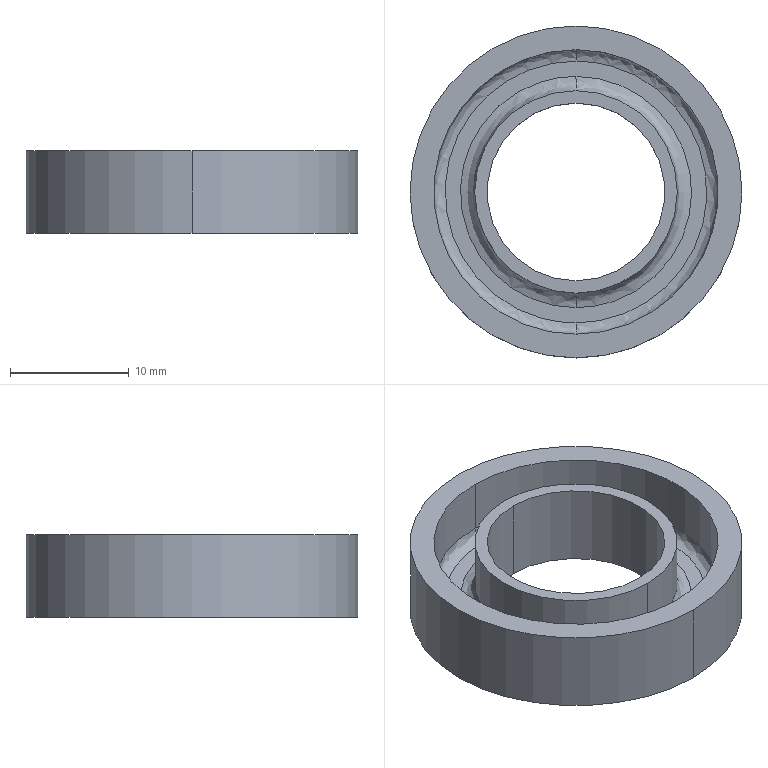Part | SolidWorks | features BaseBody 1 | 1 solid | 16 faces | box 28 x 28 x 7 mm | volume 1879 mm3 | cylinder 8 | spline 4 | plane 4 | commonest cylinder face diameters 15 x2 17.088 x2 24 x2 28 x2
STEP:
#1=CARTESIAN_POINT('',(0.,-11.038,1.5));
#2=VERTEX_POINT('',#1);
#3=CARTESIAN_POINT('',(0.,11.038,1.5));
#4=VERTEX_POINT('',#3);
#5=CARTESIAN_POINT('',(0.,-11.038,1.5));
#6=CARTESIAN_POINT('',(0.3374,-11.038,1.5));
#7=CARTESIAN_POINT('',(0.8415,-11.015,1.5));
#8=CARTESIAN_POINT('',(1.426,-10.948,1.5));
#9=CARTESIAN_POINT('',(1.718,-10.904,1.5));
#10=CARTESIAN_POINT('',(1.863,-10.879,1.5));
#11=CARTESIAN_POINT('',(1.925,-10.869,1.5));
#12=CARTESIAN_POINT('',(1.967,-10.861,1.5));
#13=CARTESIAN_POINT('',(1.986,-10.858,1.5));
#14=CARTESIAN_POINT('',(2.36,-10.788,1.5));
#15=CARTESIAN_POINT('',(2.881,-10.666,1.5));
#16=CARTESIAN_POINT('',(3.476,-10.479,1.5));
#17=CARTESIAN_POINT('',(3.771,-10.374,1.5));
#18=CARTESIAN_POINT('',(3.896,-10.327,1.5));
#19=CARTESIAN_POINT('',(3.98,-10.295,1.5));
#20=CARTESIAN_POINT('',(4.02,-10.28,1.5));
#21=CARTESIAN_POINT('',(4.41,-10.126,1.5));
#22=CARTESIAN_POINT('',(4.917,-9.895,1.5));
#23=CARTESIAN_POINT('',(5.486,-9.581,1.5));
#24=CARTESIAN_POINT('',(5.725,-9.437,1.5));
#25=CARTESIAN_POINT('',(5.883,-9.34,1.5));
#26=CARTESIAN_POINT('',(5.96,-9.291,1.5));
#27=CARTESIAN_POINT('',(6.677,-8.822,1.5));
#28=CARTESIAN_POINT('',(7.266,-8.343,1.5));
#29=CARTESIAN_POINT('',(8.074,-7.536,1.5));
#30=CARTESIAN_POINT('',(8.455,-7.113,1.5));
#31=CARTESIAN_POINT('',(8.86,-6.587,1.5));
#32=CARTESIAN_POINT('',(9.025,-6.355,1.5));
#33=CARTESIAN_POINT('',(9.133,-6.199,1.5));
#34=CARTESIAN_POINT('',(9.188,-6.118,1.5));
#35=CARTESIAN_POINT('',(9.443,-5.728,1.5));
#36=CARTESIAN_POINT('',(9.724,-5.247,1.5));
#37=CARTESIAN_POINT('',(10.008,-4.662,1.5));
#38=CARTESIAN_POINT('',(10.139,-4.365,1.5));
#39=CARTESIAN_POINT('',(10.193,-4.236,1.5));
#40=CARTESIAN_POINT('',(10.228,-4.15,1.5));
#41=CARTESIAN_POINT('',(10.246,-4.105,1.5));
#42=CARTESIAN_POINT('',(10.394,-3.73,1.5));
#43=CARTESIAN_POINT('',(10.567,-3.224,1.5));
#44=CARTESIAN_POINT('',(10.725,-2.62,1.5));
#45=CARTESIAN_POINT('',(10.793,-2.316,1.5));
#46=CARTESIAN_POINT('',(10.824,-2.162,1.5));
#47=CARTESIAN_POINT('',(10.837,-2.096,1.5));
#48=CARTESIAN_POINT('',(10.845,-2.052,1.5));
#49=CARTESIAN_POINT('',(10.85,-2.029,1.5));
#50=CARTESIAN_POINT('',(10.976,-1.345,1.5));
#51=CARTESIAN_POINT('',(11.038,-0.6753,1.5));
#52=CARTESIAN_POINT('',(11.038,0.3376,1.5));
#53=CARTESIAN_POINT('',(11.022,0.6736,1.5));
#54=CARTESIAN_POINT('',(10.976,1.176,1.5));
#55=CARTESIAN_POINT('',(10.947,1.426,1.5));
#56=CARTESIAN_POINT('',(10.904,1.718,1.5));
#57=CARTESIAN_POINT('',(10.879,1.863,1.5));
#58=CARTESIAN_POINT('',(10.868,1.925,1.5));
#59=CARTESIAN_POINT('',(10.861,1.967,1.5));
#60=CARTESIAN_POINT('',(10.858,1.986,1.5));
#61=CARTESIAN_POINT('',(10.788,2.36,1.5));
#62=CARTESIAN_POINT('',(10.666,2.881,1.5));
#63=CARTESIAN_POINT('',(10.479,3.476,1.5));
#64=CARTESIAN_POINT('',(10.374,3.771,1.5));
#65=CARTESIAN_POINT('',(10.327,3.896,1.5));
#66=CARTESIAN_POINT('',(10.295,3.98,1.5));
#67=CARTESIAN_POINT('',(10.28,4.02,1.5));
#68=CARTESIAN_POINT('',(10.126,4.41,1.5));
#69=CARTESIAN_POINT('',(9.895,4.917,1.5));
#70=CARTESIAN_POINT('',(9.581,5.486,1.5));
#71=CARTESIAN_POINT('',(9.437,5.725,1.5));
#72=CARTESIAN_POINT('',(9.34,5.883,1.5));
#73=CARTESIAN_POINT('',(9.291,5.96,1.5));
#74=CARTESIAN_POINT('',(8.822,6.677,1.5));
#75=CARTESIAN_POINT('',(8.343,7.266,1.5));
#76=CARTESIAN_POINT('',(7.536,8.074,1.5));
#77=CARTESIAN_POINT('',(7.113,8.455,1.5));
#78=CARTESIAN_POINT('',(6.587,8.86,1.5));
#79=CARTESIAN_POINT('',(6.355,9.025,1.5));
#80=CARTESIAN_POINT('',(6.199,9.133,1.5));
#81=CARTESIAN_POINT('',(6.118,9.188,1.5));
#82=CARTESIAN_POINT('',(5.728,9.443,1.5));
#83=CARTESIAN_POINT('',(5.247,9.724,1.5));
#84=CARTESIAN_POINT('',(4.662,10.008,1.5));
#85=CARTESIAN_POINT('',(4.365,10.139,1.5));
#86=CARTESIAN_POINT('',(4.236,10.193,1.5));
#87=CARTESIAN_POINT('',(4.15,10.228,1.5));
#88=CARTESIAN_POINT('',(4.105,10.246,1.5));
#89=CARTESIAN_POINT('',(3.73,10.394,1.5));
#90=CARTESIAN_POINT('',(3.224,10.567,1.5));
#91=CARTESIAN_POINT('',(2.62,10.725,1.5));
#92=CARTESIAN_POINT('',(2.316,10.793,1.5));
#93=CARTESIAN_POINT('',(2.162,10.824,1.5));
#94=CARTESIAN_POINT('',(2.096,10.837,1.5));
#95=CARTESIAN_POINT('',(2.052,10.845,1.5));
#96=CARTESIAN_POINT('',(2.029,10.85,1.5));
#97=CARTESIAN_POINT('',(1.345,10.976,1.5));
#98=CARTESIAN_POINT('',(0.6748,11.038,1.5));
#99=CARTESIAN_POINT('',(0.,11.038,1.5));
#100=B_SPLINE_CURVE_WITH_KNOTS('',3,(#5,#6,#7,#8,#9,#10,#11,#12,#13,#14,#15,#16,#17,#18,#19,#20,#21,#22,#23,#24,#25,#26,#27,#28,#29,#30,#31,#32,#33,#34,#35,#36,#37,#38,#39,#40,#41,#42,#43,#44,#45,#46,#47,#48,#49,#50,#51,#52,#53,#54,#55,#56,#57,#58,#59,#60,#61,#62,#63,#64,#65,#66,#67,#68,#69,#70,#71,#72,#73,#74,#75,#76,#77,#78,#79,#80,#81,#82,#83,#84,#85,#86,#87,#88,#89,#90,#91,#92,#93,#94,#95,#96,#97,#98,#99),.UNSPECIFIED.,.F.,.F.,(4,1,1,1,1,2,2,1,1,1,2,2,1,1,2,2,2,1,1,2,2,1,1,1,2,2,1,1,1,1,2,2,2,2,1,1,1,2,2,1,1,1,2,2,1,1,2,2,2,1,1,2,2,1,1,1,2,2,1,1,1,1,2,2,4),(0.75,0.7656,0.7734,0.7773,0.7793,0.7803,0.7812,0.7969,0.8047,0.8086,0.8105,0.8125,0.8281,0.8359,0.8398,0.8438,0.875,0.8906,0.8984,0.9023,0.9063,0.9219,0.9297,0.9336,0.9355,0.9375,0.9531,0.9609,0.9648,0.9668,0.9678,0.9688,1.,1.016,1.023,1.027,1.029,1.03,1.031,1.047,1.055,1.059,1.061,1.063,1.078,1.086,1.09,1.094,1.125,1.141,1.148,1.152,1.156,1.172,1.18,1.184,1.186,1.188,1.203,1.211,1.215,1.217,1.218,1.219,1.25),.UNSPECIFIED.);
#101=EDGE_CURVE('',#2,#4,#100,.T.);
#102=ORIENTED_EDGE('',*,*,#101,.F.);
#103=CARTESIAN_POINT('',(0.,-12.,2.462));
#104=VERTEX_POINT('',#103);
#105=CARTESIAN_POINT('',(0.,-11.038,2.462));
#106=DIRECTION('',(-1.,0.,0.));
#107=DIRECTION('',(0.,-1.,0.));
#108=AXIS2_PLACEMENT_3D('',#105,#106,#107);
#109=CIRCLE('',#108,0.9623);
#110=EDGE_CURVE('',#2,#104,#109,.T.);
#111=ORIENTED_EDGE('',*,*,#110,.T.);
#112=CARTESIAN_POINT('',(0.,12.,2.462));
#113=VERTEX_POINT('',#112);
#114=CARTESIAN_POINT('',(0.,0.,2.462));
#115=DIRECTION('',(0.,0.,1.));
#116=DIRECTION('',(0.,1.,0.));
#117=AXIS2_PLACEMENT_3D('',#114,#115,#116);
#118=CIRCLE('',#117,12.);
#119=EDGE_CURVE('',#104,#113,#118,.T.);
#120=ORIENTED_EDGE('',*,*,#119,.T.);
#121=CARTESIAN_POINT('',(0.,11.038,2.462));
#122=DIRECTION('',(1.,0.,0.));
#123=DIRECTION('',(0.,1.,0.));
#124=AXIS2_PLACEMENT_3D('',#121,#122,#123);
#125=CIRCLE('',#124,0.9623);
#126=EDGE_CURVE('',#4,#113,#125,.T.);
#127=ORIENTED_EDGE('',*,*,#126,.F.);
#128=EDGE_LOOP('',(#102,#111,#120,#127));
#129=FACE_OUTER_BOUND('',#128,.T.);
#130=CARTESIAN_POINT('',(0.,11.038,1.5));
#131=CARTESIAN_POINT('',(22.075,11.038,1.5));
#132=CARTESIAN_POINT('',(22.075,-11.038,1.5));
#133=CARTESIAN_POINT('',(0.,-11.038,1.5));
#134=CARTESIAN_POINT('',(0.,11.601,1.5));
#135=CARTESIAN_POINT('',(23.203,11.601,1.5));
#136=CARTESIAN_POINT('',(23.203,-11.601,1.5));
#137=CARTESIAN_POINT('',(0.,-11.601,1.5));
#138=CARTESIAN_POINT('',(0.,12.,1.899));
#139=CARTESIAN_POINT('',(24.,12.,1.899));
#140=CARTESIAN_POINT('',(24.,-12.,1.899));
#141=CARTESIAN_POINT('',(0.,-12.,1.899));
#142=CARTESIAN_POINT('',(0.,12.,2.462));
#143=CARTESIAN_POINT('',(24.,12.,2.462));
#144=CARTESIAN_POINT('',(24.,-12.,2.462));
#145=CARTESIAN_POINT('',(0.,-12.,2.462));
#146=(BOUNDED_SURFACE()B_SPLINE_SURFACE(3,3,((#130,#131,#132,#133),(#134,#135,#136,#137),(#138,#139,#140,#141),(#142,#143,#144,#145)),.UNSPECIFIED.,.F.,.F.,.T.)B_SPLINE_SURFACE_WITH_KNOTS((4,4),(4,4),(0.,1.),(0.,1.),.UNSPECIFIED.)GEOMETRIC_REPRESENTATION_ITEM()RATIONAL_B_SPLINE_SURFACE(((1.,0.3333,0.3333,1.),(0.8047,0.2682,0.2682,0.8047),(0.8047,0.2682,0.2682,0.8047),(1.,0.3333,0.3333,1.)))REPRESENTATION_ITEM('')SURFACE());
#147=ADVANCED_FACE('',(#129),#146,.F.);
#148=CARTESIAN_POINT('',(0.,-8.544,2.71));
#149=VERTEX_POINT('',#148);
#150=CARTESIAN_POINT('',(0.,8.544,2.71));
#151=VERTEX_POINT('',#150);
#152=CARTESIAN_POINT('',(0.,0.,2.71));
#153=DIRECTION('',(0.,0.,1.));
#154=DIRECTION('',(0.,1.,0.));
#155=AXIS2_PLACEMENT_3D('',#152,#153,#154);
#156=CIRCLE('',#155,8.544);
#157=EDGE_CURVE('',#149,#151,#156,.T.);
#158=ORIENTED_EDGE('',*,*,#157,.F.);
#159=CARTESIAN_POINT('',(0.,-9.755,1.5));
#160=VERTEX_POINT('',#159);
#161=CARTESIAN_POINT('',(0.,-9.755,2.71));
#162=DIRECTION('',(-1.,0.,0.));
#163=DIRECTION('',(0.,-1.,0.));
#164=AXIS2_PLACEMENT_3D('',#161,#162,#163);
#165=CIRCLE('',#164,1.21);
#166=EDGE_CURVE('',#149,#160,#165,.T.);
#167=ORIENTED_EDGE('',*,*,#166,.T.);
#168=CARTESIAN_POINT('',(0.,9.755,1.5));
#169=VERTEX_POINT('',#168);
#170=CARTESIAN_POINT('',(0.,9.755,1.5));
#171=CARTESIAN_POINT('',(0.2981,9.755,1.5));
#172=CARTESIAN_POINT('',(0.7436,9.734,1.5));
#173=CARTESIAN_POINT('',(1.26,9.675,1.5));
#174=CARTESIAN_POINT('',(1.518,9.636,1.5));
#175=CARTESIAN_POINT('',(1.628,9.618,1.5));
#176=CARTESIAN_POINT('',(1.702,9.605,1.5));
#177=CARTESIAN_POINT('',(1.736,9.599,1.5));
#178=CARTESIAN_POINT('',(2.086,9.534,1.5));
#179=CARTESIAN_POINT('',(2.546,9.426,1.5));
#180=CARTESIAN_POINT('',(3.072,9.261,1.5));
#181=CARTESIAN_POINT('',(3.332,9.168,1.5));
#182=CARTESIAN_POINT('',(3.443,9.127,1.5));
#183=CARTESIAN_POINT('',(3.517,9.099,1.5));
#184=CARTESIAN_POINT('',(3.552,9.085,1.5));
#185=CARTESIAN_POINT('',(3.897,8.948,1.5));
#186=CARTESIAN_POINT('',(4.345,8.744,1.5));
#187=CARTESIAN_POINT('',(4.848,8.467,1.5));
#188=CARTESIAN_POINT('',(5.059,8.34,1.5));
#189=CARTESIAN_POINT('',(5.199,8.254,1.5));
#190=CARTESIAN_POINT('',(5.267,8.211,1.5));
#191=CARTESIAN_POINT('',(5.901,7.796,1.5));
#192=CARTESIAN_POINT('',(6.422,7.373,1.5));
#193=CARTESIAN_POINT('',(7.135,6.66,1.5));
#194=CARTESIAN_POINT('',(7.472,6.286,1.5));
#195=CARTESIAN_POINT('',(7.83,5.822,1.5));
#196=CARTESIAN_POINT('',(7.976,5.616,1.5));
#197=CARTESIAN_POINT('',(8.071,5.478,1.5));
#198=CARTESIAN_POINT('',(8.119,5.407,1.5));
#199=CARTESIAN_POINT('',(8.345,5.062,1.5));
#200=CARTESIAN_POINT('',(8.593,4.637,1.5));
#201=CARTESIAN_POINT('',(8.844,4.12,1.5));
#202=CARTESIAN_POINT('',(8.96,3.857,1.5));
#203=CARTESIAN_POINT('',(9.008,3.743,1.5));
#204=CARTESIAN_POINT('',(9.039,3.667,1.5));
#205=CARTESIAN_POINT('',(9.055,3.627,1.5));
#206=CARTESIAN_POINT('',(9.186,3.297,1.5));
#207=CARTESIAN_POINT('',(9.339,2.849,1.5));
#208=CARTESIAN_POINT('',(9.478,2.316,1.5));
#209=CARTESIAN_POINT('',(9.538,2.046,1.5));
#210=CARTESIAN_POINT('',(9.566,1.911,1.5));
#211=CARTESIAN_POINT('',(9.577,1.853,1.5));
#212=CARTESIAN_POINT('',(9.584,1.814,1.5));
#213=CARTESIAN_POINT('',(9.588,1.793,1.5));
#214=CARTESIAN_POINT('',(9.7,1.188,1.5));
#215=CARTESIAN_POINT('',(9.755,0.5968,1.5));
#216=CARTESIAN_POINT('',(9.755,-0.2984,1.5));
#217=CARTESIAN_POINT('',(9.741,-0.5953,1.5));
#218=CARTESIAN_POINT('',(9.7,-1.039,1.5));
#219=CARTESIAN_POINT('',(9.675,-1.26,1.5));
#220=CARTESIAN_POINT('',(9.636,-1.518,1.5));
#221=CARTESIAN_POINT('',(9.618,-1.628,1.5));
#222=CARTESIAN_POINT('',(9.605,-1.702,1.5));
#223=CARTESIAN_POINT('',(9.599,-1.736,1.5));
#224=CARTESIAN_POINT('',(9.534,-2.086,1.5));
#225=CARTESIAN_POINT('',(9.426,-2.546,1.5));
#226=CARTESIAN_POINT('',(9.261,-3.072,1.5));
#227=CARTESIAN_POINT('',(9.168,-3.332,1.5));
#228=CARTESIAN_POINT('',(9.127,-3.443,1.5));
#229=CARTESIAN_POINT('',(9.099,-3.517,1.5));
#230=CARTESIAN_POINT('',(9.085,-3.552,1.5));
#231=CARTESIAN_POINT('',(8.948,-3.897,1.5));
#232=CARTESIAN_POINT('',(8.744,-4.345,1.5));
#233=CARTESIAN_POINT('',(8.467,-4.848,1.5));
#234=CARTESIAN_POINT('',(8.34,-5.059,1.5));
#235=CARTESIAN_POINT('',(8.254,-5.199,1.5));
#236=CARTESIAN_POINT('',(8.211,-5.267,1.5));
#237=CARTESIAN_POINT('',(7.796,-5.901,1.5));
#238=CARTESIAN_POINT('',(7.373,-6.422,1.5));
#239=CARTESIAN_POINT('',(6.66,-7.135,1.5));
#240=CARTESIAN_POINT('',(6.286,-7.472,1.5));
#241=CARTESIAN_POINT('',(5.822,-7.83,1.5));
#242=CARTESIAN_POINT('',(5.616,-7.976,1.5));
#243=CARTESIAN_POINT('',(5.478,-8.071,1.5));
#244=CARTESIAN_POINT('',(5.407,-8.119,1.5));
#245=CARTESIAN_POINT('',(5.062,-8.345,1.5));
#246=CARTESIAN_POINT('',(4.637,-8.593,1.5));
#247=CARTESIAN_POINT('',(4.12,-8.844,1.5));
#248=CARTESIAN_POINT('',(3.857,-8.96,1.5));
#249=CARTESIAN_POINT('',(3.743,-9.008,1.5));
#250=CARTESIAN_POINT('',(3.667,-9.039,1.5));
#251=CARTESIAN_POINT('',(3.627,-9.055,1.5));
#252=CARTESIAN_POINT('',(3.297,-9.186,1.5));
#253=CARTESIAN_POINT('',(2.849,-9.339,1.5));
#254=CARTESIAN_POINT('',(2.316,-9.478,1.5));
#255=CARTESIAN_POINT('',(2.046,-9.538,1.5));
#256=CARTESIAN_POINT('',(1.911,-9.566,1.5));
#257=CARTESIAN_POINT('',(1.853,-9.577,1.5));
#258=CARTESIAN_POINT('',(1.814,-9.584,1.5));
#259=CARTESIAN_POINT('',(1.793,-9.588,1.5));
#260=CARTESIAN_POINT('',(1.189,-9.7,1.5));
#261=CARTESIAN_POINT('',(0.5963,-9.754,1.5));
#262=CARTESIAN_POINT('',(0.,-9.755,1.5));
#263=B_SPLINE_CURVE_WITH_KNOTS('',3,(#170,#171,#172,#173,#174,#175,#176,#177,#178,#179,#180,#181,#182,#183,#184,#185,#186,#187,#188,#189,#190,#191,#192,#193,#194,#195,#196,#197,#198,#199,#200,#201,#202,#203,#204,#205,#206,#207,#208,#209,#210,#211,#212,#213,#214,#215,#216,#217,#218,#219,#220,#221,#222,#223,#224,#225,#226,#227,#228,#229,#230,#231,#232,#233,#234,#235,#236,#237,#238,#239,#240,#241,#242,#243,#244,#245,#246,#247,#248,#249,#250,#251,#252,#253,#254,#255,#256,#257,#258,#259,#260,#261,#262),.UNSPECIFIED.,.F.,.F.,(4,1,1,1,2,2,1,1,1,2,2,1,1,2,2,2,1,1,2,2,1,1,1,2,2,1,1,1,1,2,2,2,2,1,1,2,2,1,1,1,2,2,1,1,2,2,2,1,1,2,2,1,1,1,2,2,1,1,1,1,2,2,4),(0.75,0.7656,0.7734,0.7773,0.7793,0.7813,0.7969,0.8047,0.8086,0.8105,0.8125,0.8281,0.8359,0.8398,0.8438,0.875,0.8906,0.8984,0.9023,0.9063,0.9219,0.9297,0.9336,0.9355,0.9375,0.9531,0.9609,0.9648,0.9668,0.9678,0.9688,1.,1.016,1.023,1.027,1.029,1.031,1.047,1.055,1.059,1.061,1.063,1.078,1.086,1.09,1.094,1.125,1.141,1.148,1.152,1.156,1.172,1.18,1.184,1.186,1.188,1.203,1.211,1.215,1.217,1.218,1.219,1.25),.UNSPECIFIED.);
#264=EDGE_CURVE('',#169,#160,#263,.T.);
#265=ORIENTED_EDGE('',*,*,#264,.F.);
#266=CARTESIAN_POINT('',(0.,9.755,2.71));
#267=DIRECTION('',(1.,0.,0.));
#268=DIRECTION('',(0.,1.,0.));
#269=AXIS2_PLACEMENT_3D('',#266,#267,#268);
#270=CIRCLE('',#269,1.21);
#271=EDGE_CURVE('',#151,#169,#270,.T.);
#272=ORIENTED_EDGE('',*,*,#271,.F.);
#273=EDGE_LOOP('',(#158,#167,#265,#272));
#274=FACE_OUTER_BOUND('',#273,.T.);
#275=CARTESIAN_POINT('',(0.,8.544,2.71));
#276=CARTESIAN_POINT('',(17.088,8.544,2.71));
#277=CARTESIAN_POINT('',(17.088,-8.544,2.71));
#278=CARTESIAN_POINT('',(0.,-8.544,2.71));
#279=CARTESIAN_POINT('',(0.,8.544,2.001));
#280=CARTESIAN_POINT('',(17.088,8.544,2.001));
#281=CARTESIAN_POINT('',(17.088,-8.544,2.001));
#282=CARTESIAN_POINT('',(0.,-8.544,2.001));
#283=CARTESIAN_POINT('',(0.,9.046,1.5));
#284=CARTESIAN_POINT('',(18.091,9.046,1.5));
#285=CARTESIAN_POINT('',(18.091,-9.046,1.5));
#286=CARTESIAN_POINT('',(0.,-9.046,1.5));
#287=CARTESIAN_POINT('',(0.,9.755,1.5));
#288=CARTESIAN_POINT('',(19.509,9.755,1.5));
#289=CARTESIAN_POINT('',(19.509,-9.755,1.5));
#290=CARTESIAN_POINT('',(0.,-9.755,1.5));
#291=(BOUNDED_SURFACE()B_SPLINE_SURFACE(3,3,((#275,#276,#277,#278),(#279,#280,#281,#282),(#283,#284,#285,#286),(#287,#288,#289,#290)),.UNSPECIFIED.,.F.,.F.,.T.)B_SPLINE_SURFACE_WITH_KNOTS((4,4),(4,4),(0.,1.),(0.,1.),.UNSPECIFIED.)GEOMETRIC_REPRESENTATION_ITEM()RATIONAL_B_SPLINE_SURFACE(((1.,0.3333,0.3333,1.),(0.8047,0.2682,0.2682,0.8047),(0.8047,0.2682,0.2682,0.8047),(1.,0.3333,0.3333,1.)))REPRESENTATION_ITEM('')SURFACE());
#292=ADVANCED_FACE('',(#274),#291,.F.);
#293=CARTESIAN_POINT('',(0.,14.,7.));
#294=VERTEX_POINT('',#293);
#295=CARTESIAN_POINT('',(0.,-14.,7.));
#296=VERTEX_POINT('',#295);
#297=CARTESIAN_POINT('',(0.,0.,7.));
#298=DIRECTION('',(0.,0.,-1.));
#299=DIRECTION('',(0.,1.,0.));
#300=AXIS2_PLACEMENT_3D('',#297,#298,#299);
#301=CIRCLE('',#300,14.);
#302=EDGE_CURVE('',#294,#296,#301,.T.);
#303=ORIENTED_EDGE('',*,*,#302,.T.);
#304=CARTESIAN_POINT('',(0.,-14.,0.));
#305=VERTEX_POINT('',#304);
#306=CARTESIAN_POINT('',(0.,-14.,0.));
#307=DIRECTION('',(0.,0.,-1.));
#308=VECTOR('',#307,1000.);
#309=LINE('',#306,#308);
#310=EDGE_CURVE('',#296,#305,#309,.T.);
#311=ORIENTED_EDGE('',*,*,#310,.T.);
#312=CARTESIAN_POINT('',(0.,14.,0.));
#313=VERTEX_POINT('',#312);
#314=CARTESIAN_POINT('',(0.,0.,0.));
#315=DIRECTION('',(0.,0.,1.));
#316=DIRECTION('',(0.,1.,0.));
#317=AXIS2_PLACEMENT_3D('',#314,#315,#316);
#318=CIRCLE('',#317,14.);
#319=EDGE_CURVE('',#305,#313,#318,.T.);
#320=ORIENTED_EDGE('',*,*,#319,.T.);
#321=CARTESIAN_POINT('',(0.,14.,0.));
#322=DIRECTION('',(0.,0.,-1.));
#323=VECTOR('',#322,1000.);
#324=LINE('',#321,#323);
#325=EDGE_CURVE('',#294,#313,#324,.T.);
#326=ORIENTED_EDGE('',*,*,#325,.F.);
#327=EDGE_LOOP('',(#303,#311,#320,#326));
#328=FACE_OUTER_BOUND('',#327,.T.);
#329=CARTESIAN_POINT('',(0.,0.,0.));
#330=DIRECTION('',(0.,0.,-1.));
#331=DIRECTION('',(0.,1.,0.));
#332=AXIS2_PLACEMENT_3D('',#329,#330,#331);
#333=CYLINDRICAL_SURFACE('',#332,14.);
#334=ADVANCED_FACE('',(#328),#333,.T.);
#335=CARTESIAN_POINT('',(0.,-7.5,7.));
#336=VERTEX_POINT('',#335);
#337=CARTESIAN_POINT('',(0.,7.5,7.));
#338=VERTEX_POINT('',#337);
#339=CARTESIAN_POINT('',(0.,0.,7.));
#340=DIRECTION('',(0.,0.,-1.));
#341=DIRECTION('',(0.,1.,0.));
#342=AXIS2_PLACEMENT_3D('',#339,#340,#341);
#343=CIRCLE('',#342,7.5);
#344=EDGE_CURVE('',#336,#338,#343,.T.);
#345=ORIENTED_EDGE('',*,*,#344,.F.);
#346=CARTESIAN_POINT('',(0.,-7.5,0.));
#347=VERTEX_POINT('',#346);
#348=CARTESIAN_POINT('',(0.,-7.5,0.));
#349=DIRECTION('',(0.,0.,-1.));
#350=VECTOR('',#349,1000.);
#351=LINE('',#348,#350);
#352=EDGE_CURVE('',#336,#347,#351,.T.);
#353=ORIENTED_EDGE('',*,*,#352,.T.);
#354=CARTESIAN_POINT('',(0.,7.5,0.));
#355=VERTEX_POINT('',#354);
#356=CARTESIAN_POINT('',(0.,0.,0.));
#357=DIRECTION('',(0.,0.,1.));
#358=DIRECTION('',(0.,1.,0.));
#359=AXIS2_PLACEMENT_3D('',#356,#357,#358);
#360=CIRCLE('',#359,7.5);
#361=EDGE_CURVE('',#355,#347,#360,.T.);
#362=ORIENTED_EDGE('',*,*,#361,.F.);
#363=CARTESIAN_POINT('',(0.,7.5,0.));
#364=DIRECTION('',(0.,0.,-1.));
#365=VECTOR('',#364,1000.);
#366=LINE('',#363,#365);
#367=EDGE_CURVE('',#338,#355,#366,.T.);
#368=ORIENTED_EDGE('',*,*,#367,.F.);
#369=EDGE_LOOP('',(#345,#353,#362,#368));
#370=FACE_OUTER_BOUND('',#369,.T.);
#371=CARTESIAN_POINT('',(0.,0.,0.));
#372=DIRECTION('',(0.,0.,-1.));
#373=DIRECTION('',(0.,1.,0.));
#374=AXIS2_PLACEMENT_3D('',#371,#372,#373);
#375=CYLINDRICAL_SURFACE('',#374,7.5);
#376=ADVANCED_FACE('',(#370),#375,.F.);
#377=CARTESIAN_POINT('',(0.,-12.,7.));
#378=VERTEX_POINT('',#377);
#379=CARTESIAN_POINT('',(0.,12.,7.));
#380=VERTEX_POINT('',#379);
#381=CARTESIAN_POINT('',(0.,0.,7.));
#382=DIRECTION('',(0.,0.,-1.));
#383=DIRECTION('',(0.,1.,0.));
#384=AXIS2_PLACEMENT_3D('',#381,#382,#383);
#385=CIRCLE('',#384,12.);
#386=EDGE_CURVE('',#378,#380,#385,.T.);
#387=ORIENTED_EDGE('',*,*,#386,.F.);
#388=CARTESIAN_POINT('',(0.,-12.,0.));
#389=DIRECTION('',(0.,0.,-1.));
#390=VECTOR('',#389,1000.);
#391=LINE('',#388,#390);
#392=EDGE_CURVE('',#378,#104,#391,.T.);
#393=ORIENTED_EDGE('',*,*,#392,.T.);
#394=CARTESIAN_POINT('',(0.,0.,2.462));
#395=DIRECTION('',(0.,0.,1.));
#396=DIRECTION('',(0.,1.,0.));
#397=AXIS2_PLACEMENT_3D('',#394,#395,#396);
#398=CIRCLE('',#397,12.);
#399=EDGE_CURVE('',#113,#104,#398,.T.);
#400=ORIENTED_EDGE('',*,*,#399,.F.);
#401=CARTESIAN_POINT('',(0.,12.,0.));
#402=DIRECTION('',(0.,0.,-1.));
#403=VECTOR('',#402,1000.);
#404=LINE('',#401,#403);
#405=EDGE_CURVE('',#380,#113,#404,.T.);
#406=ORIENTED_EDGE('',*,*,#405,.F.);
#407=EDGE_LOOP('',(#387,#393,#400,#406));
#408=FACE_OUTER_BOUND('',#407,.T.);
#409=CARTESIAN_POINT('',(0.,0.,0.));
#410=DIRECTION('',(0.,0.,-1.));
#411=DIRECTION('',(0.,1.,0.));
#412=AXIS2_PLACEMENT_3D('',#409,#410,#411);
#413=CYLINDRICAL_SURFACE('',#412,12.);
#414=ADVANCED_FACE('',(#408),#413,.F.);
#415=CARTESIAN_POINT('',(0.,-8.544,7.));
#416=VERTEX_POINT('',#415);
#417=CARTESIAN_POINT('',(0.,8.544,7.));
#418=VERTEX_POINT('',#417);
#419=CARTESIAN_POINT('',(0.,0.,7.));
#420=DIRECTION('',(0.,0.,1.));
#421=DIRECTION('',(0.,1.,0.));
#422=AXIS2_PLACEMENT_3D('',#419,#420,#421);
#423=CIRCLE('',#422,8.544);
#424=EDGE_CURVE('',#416,#418,#423,.T.);
#425=ORIENTED_EDGE('',*,*,#424,.F.);
#426=CARTESIAN_POINT('',(0.,-8.544,0.));
#427=DIRECTION('',(0.,0.,-1.));
#428=VECTOR('',#427,1000.);
#429=LINE('',#426,#428);
#430=EDGE_CURVE('',#416,#149,#429,.T.);
#431=ORIENTED_EDGE('',*,*,#430,.T.);
#432=ORIENTED_EDGE('',*,*,#157,.T.);
#433=CARTESIAN_POINT('',(0.,8.544,0.));
#434=DIRECTION('',(0.,0.,-1.));
#435=VECTOR('',#434,1000.);
#436=LINE('',#433,#435);
#437=EDGE_CURVE('',#418,#151,#436,.T.);
#438=ORIENTED_EDGE('',*,*,#437,.F.);
#439=EDGE_LOOP('',(#425,#431,#432,#438));
#440=FACE_OUTER_BOUND('',#439,.T.);
#441=CARTESIAN_POINT('',(0.,0.,0.));
#442=DIRECTION('',(0.,0.,-1.));
#443=DIRECTION('',(0.,1.,0.));
#444=AXIS2_PLACEMENT_3D('',#441,#442,#443);
#445=CYLINDRICAL_SURFACE('',#444,8.544);
#446=ADVANCED_FACE('',(#440),#445,.T.);
#447=ORIENTED_EDGE('',*,*,#310,.F.);
#448=CARTESIAN_POINT('',(0.,0.,7.));
#449=DIRECTION('',(0.,0.,-1.));
#450=DIRECTION('',(0.,1.,0.));
#451=AXIS2_PLACEMENT_3D('',#448,#449,#450);
#452=CIRCLE('',#451,14.);
#453=EDGE_CURVE('',#296,#294,#452,.T.);
#454=ORIENTED_EDGE('',*,*,#453,.T.);
#455=ORIENTED_EDGE('',*,*,#325,.T.);
#456=CARTESIAN_POINT('',(0.,0.,0.));
#457=DIRECTION('',(0.,0.,1.));
#458=DIRECTION('',(0.,1.,0.));
#459=AXIS2_PLACEMENT_3D('',#456,#457,#458);
#460=CIRCLE('',#459,14.);
#461=EDGE_CURVE('',#313,#305,#460,.T.);
#462=ORIENTED_EDGE('',*,*,#461,.T.);
#463=EDGE_LOOP('',(#447,#454,#455,#462));
#464=FACE_OUTER_BOUND('',#463,.T.);
#465=CARTESIAN_POINT('',(0.,0.,0.));
#466=DIRECTION('',(0.,0.,-1.));
#467=DIRECTION('',(0.,1.,0.));
#468=AXIS2_PLACEMENT_3D('',#465,#466,#467);
#469=CYLINDRICAL_SURFACE('',#468,14.);
#470=ADVANCED_FACE('',(#464),#469,.T.);
#471=ORIENTED_EDGE('',*,*,#361,.T.);
#472=CARTESIAN_POINT('',(0.,0.,0.));
#473=DIRECTION('',(0.,0.,1.));
#474=DIRECTION('',(0.,1.,0.));
#475=AXIS2_PLACEMENT_3D('',#472,#473,#474);
#476=CIRCLE('',#475,7.5);
#477=EDGE_CURVE('',#347,#355,#476,.T.);
#478=ORIENTED_EDGE('',*,*,#477,.T.);
#479=EDGE_LOOP('',(#471,#478));
#480=FACE_BOUND('',#479,.T.);
#481=ORIENTED_EDGE('',*,*,#461,.F.);
#482=ORIENTED_EDGE('',*,*,#319,.F.);
#483=EDGE_LOOP('',(#481,#482));
#484=FACE_OUTER_BOUND('',#483,.T.);
#485=CARTESIAN_POINT('',(7.5,0.,0.));
#486=DIRECTION('',(0.,0.,-1.));
#487=DIRECTION('',(0.,1.,0.));
#488=AXIS2_PLACEMENT_3D('',#485,#486,#487);
#489=PLANE('',#488);
#490=ADVANCED_FACE('',(#480,#484),#489,.T.);
#491=ORIENTED_EDGE('',*,*,#302,.F.);
#492=ORIENTED_EDGE('',*,*,#453,.F.);
#493=EDGE_LOOP('',(#491,#492));
#494=FACE_OUTER_BOUND('',#493,.T.);
#495=CARTESIAN_POINT('',(0.,0.,7.));
#496=DIRECTION('',(0.,0.,-1.));
#497=DIRECTION('',(0.,1.,0.));
#498=AXIS2_PLACEMENT_3D('',#495,#496,#497);
#499=CIRCLE('',#498,12.);
#500=EDGE_CURVE('',#380,#378,#499,.T.);
#501=ORIENTED_EDGE('',*,*,#500,.T.);
#502=ORIENTED_EDGE('',*,*,#386,.T.);
#503=EDGE_LOOP('',(#501,#502));
#504=FACE_BOUND('',#503,.T.);
#505=CARTESIAN_POINT('',(14.,0.,7.));
#506=DIRECTION('',(0.,0.,1.));
#507=DIRECTION('',(0.,-1.,0.));
#508=AXIS2_PLACEMENT_3D('',#505,#506,#507);
#509=PLANE('',#508);
#510=ADVANCED_FACE('',(#494,#504),#509,.T.);
#511=ORIENTED_EDGE('',*,*,#352,.F.);
#512=CARTESIAN_POINT('',(0.,0.,7.));
#513=DIRECTION('',(0.,0.,-1.));
#514=DIRECTION('',(0.,1.,0.));
#515=AXIS2_PLACEMENT_3D('',#512,#513,#514);
#516=CIRCLE('',#515,7.5);
#517=EDGE_CURVE('',#338,#336,#516,.T.);
#518=ORIENTED_EDGE('',*,*,#517,.F.);
#519=ORIENTED_EDGE('',*,*,#367,.T.);
#520=ORIENTED_EDGE('',*,*,#477,.F.);
#521=EDGE_LOOP('',(#511,#518,#519,#520));
#522=FACE_OUTER_BOUND('',#521,.T.);
#523=CARTESIAN_POINT('',(0.,0.,0.));
#524=DIRECTION('',(0.,0.,-1.));
#525=DIRECTION('',(0.,1.,0.));
#526=AXIS2_PLACEMENT_3D('',#523,#524,#525);
#527=CYLINDRICAL_SURFACE('',#526,7.5);
#528=ADVANCED_FACE('',(#522),#527,.F.);
#529=ORIENTED_EDGE('',*,*,#392,.F.);
#530=ORIENTED_EDGE('',*,*,#500,.F.);
#531=ORIENTED_EDGE('',*,*,#405,.T.);
#532=ORIENTED_EDGE('',*,*,#119,.F.);
#533=EDGE_LOOP('',(#529,#530,#531,#532));
#534=FACE_OUTER_BOUND('',#533,.T.);
#535=CARTESIAN_POINT('',(0.,0.,0.));
#536=DIRECTION('',(0.,0.,-1.));
#537=DIRECTION('',(0.,1.,0.));
#538=AXIS2_PLACEMENT_3D('',#535,#536,#537);
#539=CYLINDRICAL_SURFACE('',#538,12.);
#540=ADVANCED_FACE('',(#534),#539,.F.);
#541=CARTESIAN_POINT('',(0.,0.,7.));
#542=DIRECTION('',(0.,0.,1.));
#543=DIRECTION('',(0.,1.,0.));
#544=AXIS2_PLACEMENT_3D('',#541,#542,#543);
#545=CIRCLE('',#544,8.544);
#546=EDGE_CURVE('',#418,#416,#545,.T.);
#547=ORIENTED_EDGE('',*,*,#546,.T.);
#548=ORIENTED_EDGE('',*,*,#424,.T.);
#549=EDGE_LOOP('',(#547,#548));
#550=FACE_OUTER_BOUND('',#549,.T.);
#551=ORIENTED_EDGE('',*,*,#517,.T.);
#552=ORIENTED_EDGE('',*,*,#344,.T.);
#553=EDGE_LOOP('',(#551,#552));
#554=FACE_BOUND('',#553,.T.);
#555=CARTESIAN_POINT('',(8.544,0.,7.));
#556=DIRECTION('',(0.,0.,1.));
#557=DIRECTION('',(0.,-1.,0.));
#558=AXIS2_PLACEMENT_3D('',#555,#556,#557);
#559=PLANE('',#558);
#560=ADVANCED_FACE('',(#550,#554),#559,.T.);
#561=ORIENTED_EDGE('',*,*,#110,.F.);
#562=CARTESIAN_POINT('',(0.,11.038,1.5));
#563=CARTESIAN_POINT('',(-0.3374,11.038,1.5));
#564=CARTESIAN_POINT('',(-0.8415,11.015,1.5));
#565=CARTESIAN_POINT('',(-1.426,10.948,1.5));
#566=CARTESIAN_POINT('',(-1.718,10.904,1.5));
#567=CARTESIAN_POINT('',(-1.863,10.879,1.5));
#568=CARTESIAN_POINT('',(-1.925,10.869,1.5));
#569=CARTESIAN_POINT('',(-1.967,10.861,1.5));
#570=CARTESIAN_POINT('',(-1.986,10.858,1.5));
#571=CARTESIAN_POINT('',(-2.36,10.788,1.5));
#572=CARTESIAN_POINT('',(-2.881,10.666,1.5));
#573=CARTESIAN_POINT('',(-3.476,10.479,1.5));
#574=CARTESIAN_POINT('',(-3.771,10.374,1.5));
#575=CARTESIAN_POINT('',(-3.896,10.327,1.5));
#576=CARTESIAN_POINT('',(-3.98,10.295,1.5));
#577=CARTESIAN_POINT('',(-4.02,10.28,1.5));
#578=CARTESIAN_POINT('',(-4.41,10.126,1.5));
#579=CARTESIAN_POINT('',(-4.917,9.895,1.5));
#580=CARTESIAN_POINT('',(-5.486,9.581,1.5));
#581=CARTESIAN_POINT('',(-5.725,9.437,1.5));
#582=CARTESIAN_POINT('',(-5.883,9.34,1.5));
#583=CARTESIAN_POINT('',(-5.96,9.291,1.5));
#584=CARTESIAN_POINT('',(-6.677,8.822,1.5));
#585=CARTESIAN_POINT('',(-7.266,8.343,1.5));
#586=CARTESIAN_POINT('',(-8.074,7.536,1.5));
#587=CARTESIAN_POINT('',(-8.455,7.113,1.5));
#588=CARTESIAN_POINT('',(-8.86,6.587,1.5));
#589=CARTESIAN_POINT('',(-9.025,6.355,1.5));
#590=CARTESIAN_POINT('',(-9.133,6.199,1.5));
#591=CARTESIAN_POINT('',(-9.188,6.118,1.5));
#592=CARTESIAN_POINT('',(-9.443,5.728,1.5));
#593=CARTESIAN_POINT('',(-9.724,5.247,1.5));
#594=CARTESIAN_POINT('',(-10.008,4.662,1.5));
#595=CARTESIAN_POINT('',(-10.139,4.365,1.5));
#596=CARTESIAN_POINT('',(-10.193,4.236,1.5));
#597=CARTESIAN_POINT('',(-10.228,4.15,1.5));
#598=CARTESIAN_POINT('',(-10.246,4.105,1.5));
#599=CARTESIAN_POINT('',(-10.394,3.73,1.5));
#600=CARTESIAN_POINT('',(-10.567,3.224,1.5));
#601=CARTESIAN_POINT('',(-10.725,2.62,1.5));
#602=CARTESIAN_POINT('',(-10.793,2.316,1.5));
#603=CARTESIAN_POINT('',(-10.824,2.162,1.5));
#604=CARTESIAN_POINT('',(-10.837,2.096,1.5));
#605=CARTESIAN_POINT('',(-10.845,2.052,1.5));
#606=CARTESIAN_POINT('',(-10.85,2.029,1.5));
#607=CARTESIAN_POINT('',(-10.976,1.345,1.5));
#608=CARTESIAN_POINT('',(-11.038,0.6748,1.5));
#609=CARTESIAN_POINT('',(-11.038,-0.3374,1.5));
#610=CARTESIAN_POINT('',(-11.015,-0.8415,1.5));
#611=CARTESIAN_POINT('',(-10.948,-1.426,1.5));
#612=CARTESIAN_POINT('',(-10.904,-1.718,1.5));
#613=CARTESIAN_POINT('',(-10.879,-1.863,1.5));
#614=CARTESIAN_POINT('',(-10.869,-1.925,1.5));
#615=CARTESIAN_POINT('',(-10.861,-1.967,1.5));
#616=CARTESIAN_POINT('',(-10.858,-1.986,1.5));
#617=CARTESIAN_POINT('',(-10.788,-2.36,1.5));
#618=CARTESIAN_POINT('',(-10.666,-2.881,1.5));
#619=CARTESIAN_POINT('',(-10.479,-3.476,1.5));
#620=CARTESIAN_POINT('',(-10.374,-3.771,1.5));
#621=CARTESIAN_POINT('',(-10.327,-3.896,1.5));
#622=CARTESIAN_POINT('',(-10.295,-3.98,1.5));
#623=CARTESIAN_POINT('',(-10.28,-4.02,1.5));
#624=CARTESIAN_POINT('',(-10.126,-4.41,1.5));
#625=CARTESIAN_POINT('',(-9.895,-4.917,1.5));
#626=CARTESIAN_POINT('',(-9.581,-5.486,1.5));
#627=CARTESIAN_POINT('',(-9.437,-5.725,1.5));
#628=CARTESIAN_POINT('',(-9.34,-5.883,1.5));
#629=CARTESIAN_POINT('',(-9.291,-5.96,1.5));
#630=CARTESIAN_POINT('',(-8.822,-6.677,1.5));
#631=CARTESIAN_POINT('',(-8.343,-7.266,1.5));
#632=CARTESIAN_POINT('',(-7.536,-8.074,1.5));
#633=CARTESIAN_POINT('',(-7.113,-8.455,1.5));
#634=CARTESIAN_POINT('',(-6.587,-8.86,1.5));
#635=CARTESIAN_POINT('',(-6.355,-9.025,1.5));
#636=CARTESIAN_POINT('',(-6.199,-9.133,1.5));
#637=CARTESIAN_POINT('',(-6.118,-9.188,1.5));
#638=CARTESIAN_POINT('',(-5.728,-9.443,1.5));
#639=CARTESIAN_POINT('',(-5.247,-9.724,1.5));
#640=CARTESIAN_POINT('',(-4.662,-10.008,1.5));
#641=CARTESIAN_POINT('',(-4.365,-10.139,1.5));
#642=CARTESIAN_POINT('',(-4.236,-10.193,1.5));
#643=CARTESIAN_POINT('',(-4.15,-10.228,1.5));
#644=CARTESIAN_POINT('',(-4.105,-10.246,1.5));
#645=CARTESIAN_POINT('',(-3.73,-10.394,1.5));
#646=CARTESIAN_POINT('',(-3.224,-10.567,1.5));
#647=CARTESIAN_POINT('',(-2.62,-10.725,1.5));
#648=CARTESIAN_POINT('',(-2.316,-10.793,1.5));
#649=CARTESIAN_POINT('',(-2.162,-10.824,1.5));
#650=CARTESIAN_POINT('',(-2.096,-10.837,1.5));
#651=CARTESIAN_POINT('',(-2.052,-10.845,1.5));
#652=CARTESIAN_POINT('',(-2.029,-10.85,1.5));
#653=CARTESIAN_POINT('',(-1.345,-10.976,1.5));
#654=CARTESIAN_POINT('',(-0.6748,-11.038,1.5));
#655=CARTESIAN_POINT('',(0.,-11.038,1.5));
#656=B_SPLINE_CURVE_WITH_KNOTS('',3,(#562,#563,#564,#565,#566,#567,#568,#569,#570,#571,#572,#573,#574,#575,#576,#577,#578,#579,#580,#581,#582,#583,#584,#585,#586,#587,#588,#589,#590,#591,#592,#593,#594,#595,#596,#597,#598,#599,#600,#601,#602,#603,#604,#605,#606,#607,#608,#609,#610,#611,#612,#613,#614,#615,#616,#617,#618,#619,#620,#621,#622,#623,#624,#625,#626,#627,#628,#629,#630,#631,#632,#633,#634,#635,#636,#637,#638,#639,#640,#641,#642,#643,#644,#645,#646,#647,#648,#649,#650,#651,#652,#653,#654,#655),.UNSPECIFIED.,.F.,.F.,(4,1,1,1,1,2,2,1,1,1,2,2,1,1,2,2,2,1,1,2,2,1,1,1,2,2,1,1,1,1,2,2,2,1,1,1,1,2,2,1,1,1,2,2,1,1,2,2,2,1,1,2,2,1,1,1,2,2,1,1,1,1,2,2,4),(0.25,0.2656,0.2734,0.2773,0.2793,0.2803,0.2813,0.2969,0.3047,0.3086,0.3105,0.3125,0.3281,0.3359,0.3398,0.3438,0.375,0.3906,0.3984,0.4023,0.4063,0.4219,0.4297,0.4336,0.4355,0.4375,0.4531,0.4609,0.4648,0.4668,0.4678,0.4688,0.5,0.5156,0.5234,0.5273,0.5293,0.5303,0.5313,0.5469,0.5547,0.5586,0.5605,0.5625,0.5781,0.5859,0.5898,0.5938,0.625,0.6406,0.6484,0.6523,0.6563,0.6719,0.6797,0.6836,0.6855,0.6875,0.7031,0.7109,0.7148,0.7168,0.7178,0.7188,0.75),.UNSPECIFIED.);
#657=EDGE_CURVE('',#4,#2,#656,.T.);
#658=ORIENTED_EDGE('',*,*,#657,.F.);
#659=ORIENTED_EDGE('',*,*,#126,.T.);
#660=ORIENTED_EDGE('',*,*,#399,.T.);
#661=EDGE_LOOP('',(#561,#658,#659,#660));
#662=FACE_OUTER_BOUND('',#661,.T.);
#663=CARTESIAN_POINT('',(0.,-11.038,1.5));
#664=CARTESIAN_POINT('',(-22.075,-11.038,1.5));
#665=CARTESIAN_POINT('',(-22.075,11.038,1.5));
#666=CARTESIAN_POINT('',(0.,11.038,1.5));
#667=CARTESIAN_POINT('',(0.,-11.601,1.5));
#668=CARTESIAN_POINT('',(-23.203,-11.601,1.5));
#669=CARTESIAN_POINT('',(-23.203,11.601,1.5));
#670=CARTESIAN_POINT('',(0.,11.601,1.5));
#671=CARTESIAN_POINT('',(0.,-12.,1.899));
#672=CARTESIAN_POINT('',(-24.,-12.,1.899));
#673=CARTESIAN_POINT('',(-24.,12.,1.899));
#674=CARTESIAN_POINT('',(0.,12.,1.899));
#675=CARTESIAN_POINT('',(0.,-12.,2.462));
#676=CARTESIAN_POINT('',(-24.,-12.,2.462));
#677=CARTESIAN_POINT('',(-24.,12.,2.462));
#678=CARTESIAN_POINT('',(0.,12.,2.462));
#679=(BOUNDED_SURFACE()B_SPLINE_SURFACE(3,3,((#663,#664,#665,#666),(#667,#668,#669,#670),(#671,#672,#673,#674),(#675,#676,#677,#678)),.UNSPECIFIED.,.F.,.F.,.F.)B_SPLINE_SURFACE_WITH_KNOTS((4,4),(4,4),(0.,1.),(0.,1.),.UNSPECIFIED.)GEOMETRIC_REPRESENTATION_ITEM()RATIONAL_B_SPLINE_SURFACE(((1.,0.3333,0.3333,1.),(0.8047,0.2682,0.2682,0.8047),(0.8047,0.2682,0.2682,0.8047),(1.,0.3333,0.3333,1.)))REPRESENTATION_ITEM('')SURFACE());
#680=ADVANCED_FACE('',(#662),#679,.F.);
#681=ORIENTED_EDGE('',*,*,#430,.F.);
#682=ORIENTED_EDGE('',*,*,#546,.F.);
#683=ORIENTED_EDGE('',*,*,#437,.T.);
#684=CARTESIAN_POINT('',(0.,0.,2.71));
#685=DIRECTION('',(0.,0.,1.));
#686=DIRECTION('',(0.,1.,0.));
#687=AXIS2_PLACEMENT_3D('',#684,#685,#686);
#688=CIRCLE('',#687,8.544);
#689=EDGE_CURVE('',#151,#149,#688,.T.);
#690=ORIENTED_EDGE('',*,*,#689,.T.);
#691=EDGE_LOOP('',(#681,#682,#683,#690));
#692=FACE_OUTER_BOUND('',#691,.T.);
#693=CARTESIAN_POINT('',(0.,0.,0.));
#694=DIRECTION('',(0.,0.,-1.));
#695=DIRECTION('',(0.,1.,0.));
#696=AXIS2_PLACEMENT_3D('',#693,#694,#695);
#697=CYLINDRICAL_SURFACE('',#696,8.544);
#698=ADVANCED_FACE('',(#692),#697,.T.);
#699=ORIENTED_EDGE('',*,*,#657,.T.);
#700=ORIENTED_EDGE('',*,*,#101,.T.);
#701=EDGE_LOOP('',(#699,#700));
#702=FACE_OUTER_BOUND('',#701,.T.);
#703=ORIENTED_EDGE('',*,*,#264,.T.);
#704=CARTESIAN_POINT('',(0.,-9.755,1.5));
#705=CARTESIAN_POINT('',(-0.2981,-9.755,1.5));
#706=CARTESIAN_POINT('',(-0.7436,-9.734,1.5));
#707=CARTESIAN_POINT('',(-1.26,-9.675,1.5));
#708=CARTESIAN_POINT('',(-1.518,-9.636,1.5));
#709=CARTESIAN_POINT('',(-1.628,-9.618,1.5));
#710=CARTESIAN_POINT('',(-1.702,-9.605,1.5));
#711=CARTESIAN_POINT('',(-1.736,-9.599,1.5));
#712=CARTESIAN_POINT('',(-2.086,-9.534,1.5));
#713=CARTESIAN_POINT('',(-2.546,-9.426,1.5));
#714=CARTESIAN_POINT('',(-3.072,-9.261,1.5));
#715=CARTESIAN_POINT('',(-3.332,-9.168,1.5));
#716=CARTESIAN_POINT('',(-3.443,-9.127,1.5));
#717=CARTESIAN_POINT('',(-3.517,-9.099,1.5));
#718=CARTESIAN_POINT('',(-3.552,-9.085,1.5));
#719=CARTESIAN_POINT('',(-3.897,-8.948,1.5));
#720=CARTESIAN_POINT('',(-4.345,-8.744,1.5));
#721=CARTESIAN_POINT('',(-4.848,-8.467,1.5));
#722=CARTESIAN_POINT('',(-5.059,-8.34,1.5));
#723=CARTESIAN_POINT('',(-5.199,-8.254,1.5));
#724=CARTESIAN_POINT('',(-5.267,-8.211,1.5));
#725=CARTESIAN_POINT('',(-5.901,-7.796,1.5));
#726=CARTESIAN_POINT('',(-6.422,-7.373,1.5));
#727=CARTESIAN_POINT('',(-7.135,-6.66,1.5));
#728=CARTESIAN_POINT('',(-7.472,-6.286,1.5));
#729=CARTESIAN_POINT('',(-7.83,-5.822,1.5));
#730=CARTESIAN_POINT('',(-7.976,-5.616,1.5));
#731=CARTESIAN_POINT('',(-8.071,-5.478,1.5));
#732=CARTESIAN_POINT('',(-8.119,-5.407,1.5));
#733=CARTESIAN_POINT('',(-8.345,-5.062,1.5));
#734=CARTESIAN_POINT('',(-8.593,-4.637,1.5));
#735=CARTESIAN_POINT('',(-8.844,-4.12,1.5));
#736=CARTESIAN_POINT('',(-8.96,-3.857,1.5));
#737=CARTESIAN_POINT('',(-9.008,-3.743,1.5));
#738=CARTESIAN_POINT('',(-9.039,-3.667,1.5));
#739=CARTESIAN_POINT('',(-9.055,-3.627,1.5));
#740=CARTESIAN_POINT('',(-9.186,-3.297,1.5));
#741=CARTESIAN_POINT('',(-9.339,-2.849,1.5));
#742=CARTESIAN_POINT('',(-9.478,-2.316,1.5));
#743=CARTESIAN_POINT('',(-9.538,-2.046,1.5));
#744=CARTESIAN_POINT('',(-9.566,-1.911,1.5));
#745=CARTESIAN_POINT('',(-9.577,-1.853,1.5));
#746=CARTESIAN_POINT('',(-9.584,-1.814,1.5));
#747=CARTESIAN_POINT('',(-9.588,-1.793,1.5));
#748=CARTESIAN_POINT('',(-9.7,-1.189,1.5));
#749=CARTESIAN_POINT('',(-9.754,-0.5963,1.5));
#750=CARTESIAN_POINT('',(-9.755,0.2981,1.5));
#751=CARTESIAN_POINT('',(-9.734,0.7436,1.5));
#752=CARTESIAN_POINT('',(-9.675,1.26,1.5));
#753=CARTESIAN_POINT('',(-9.636,1.518,1.5));
#754=CARTESIAN_POINT('',(-9.618,1.628,1.5));
#755=CARTESIAN_POINT('',(-9.605,1.702,1.5));
#756=CARTESIAN_POINT('',(-9.599,1.736,1.5));
#757=CARTESIAN_POINT('',(-9.534,2.086,1.5));
#758=CARTESIAN_POINT('',(-9.426,2.546,1.5));
#759=CARTESIAN_POINT('',(-9.261,3.072,1.5));
#760=CARTESIAN_POINT('',(-9.168,3.332,1.5));
#761=CARTESIAN_POINT('',(-9.127,3.443,1.5));
#762=CARTESIAN_POINT('',(-9.099,3.517,1.5));
#763=CARTESIAN_POINT('',(-9.085,3.552,1.5));
#764=CARTESIAN_POINT('',(-8.948,3.897,1.5));
#765=CARTESIAN_POINT('',(-8.744,4.345,1.5));
#766=CARTESIAN_POINT('',(-8.467,4.848,1.5));
#767=CARTESIAN_POINT('',(-8.34,5.059,1.5));
#768=CARTESIAN_POINT('',(-8.254,5.199,1.5));
#769=CARTESIAN_POINT('',(-8.211,5.267,1.5));
#770=CARTESIAN_POINT('',(-7.796,5.901,1.5));
#771=CARTESIAN_POINT('',(-7.373,6.422,1.5));
#772=CARTESIAN_POINT('',(-6.66,7.135,1.5));
#773=CARTESIAN_POINT('',(-6.286,7.472,1.5));
#774=CARTESIAN_POINT('',(-5.822,7.83,1.5));
#775=CARTESIAN_POINT('',(-5.616,7.976,1.5));
#776=CARTESIAN_POINT('',(-5.478,8.071,1.5));
#777=CARTESIAN_POINT('',(-5.407,8.119,1.5));
#778=CARTESIAN_POINT('',(-5.062,8.345,1.5));
#779=CARTESIAN_POINT('',(-4.637,8.593,1.5));
#780=CARTESIAN_POINT('',(-4.12,8.844,1.5));
#781=CARTESIAN_POINT('',(-3.857,8.96,1.5));
#782=CARTESIAN_POINT('',(-3.743,9.008,1.5));
#783=CARTESIAN_POINT('',(-3.667,9.039,1.5));
#784=CARTESIAN_POINT('',(-3.627,9.055,1.5));
#785=CARTESIAN_POINT('',(-3.297,9.186,1.5));
#786=CARTESIAN_POINT('',(-2.849,9.339,1.5));
#787=CARTESIAN_POINT('',(-2.316,9.478,1.5));
#788=CARTESIAN_POINT('',(-2.046,9.538,1.5));
#789=CARTESIAN_POINT('',(-1.911,9.566,1.5));
#790=CARTESIAN_POINT('',(-1.853,9.577,1.5));
#791=CARTESIAN_POINT('',(-1.814,9.584,1.5));
#792=CARTESIAN_POINT('',(-1.793,9.588,1.5));
#793=CARTESIAN_POINT('',(-1.189,9.7,1.5));
#794=CARTESIAN_POINT('',(-0.5963,9.754,1.5));
#795=CARTESIAN_POINT('',(0.,9.755,1.5));
#796=B_SPLINE_CURVE_WITH_KNOTS('',3,(#704,#705,#706,#707,#708,#709,#710,#711,#712,#713,#714,#715,#716,#717,#718,#719,#720,#721,#722,#723,#724,#725,#726,#727,#728,#729,#730,#731,#732,#733,#734,#735,#736,#737,#738,#739,#740,#741,#742,#743,#744,#745,#746,#747,#748,#749,#750,#751,#752,#753,#754,#755,#756,#757,#758,#759,#760,#761,#762,#763,#764,#765,#766,#767,#768,#769,#770,#771,#772,#773,#774,#775,#776,#777,#778,#779,#780,#781,#782,#783,#784,#785,#786,#787,#788,#789,#790,#791,#792,#793,#794,#795),.UNSPECIFIED.,.F.,.F.,(4,1,1,1,2,2,1,1,1,2,2,1,1,2,2,2,1,1,2,2,1,1,1,2,2,1,1,1,1,2,2,2,1,1,1,2,2,1,1,1,2,2,1,1,2,2,2,1,1,2,2,1,1,1,2,2,1,1,1,1,2,2,4),(0.25,0.2656,0.2734,0.2773,0.2793,0.2812,0.2969,0.3047,0.3086,0.3105,0.3125,0.3281,0.3359,0.3398,0.3437,0.375,0.3906,0.3984,0.4023,0.4062,0.4219,0.4297,0.4336,0.4355,0.4375,0.4531,0.4609,0.4648,0.4668,0.4678,0.4687,0.5,0.5156,0.5234,0.5273,0.5293,0.5312,0.5469,0.5547,0.5586,0.5605,0.5625,0.5781,0.5859,0.5898,0.5937,0.625,0.6406,0.6484,0.6523,0.6562,0.6719,0.6797,0.6836,0.6855,0.6875,0.7031,0.7109,0.7148,0.7168,0.7178,0.7187,0.75),.UNSPECIFIED.);
#797=EDGE_CURVE('',#160,#169,#796,.T.);
#798=ORIENTED_EDGE('',*,*,#797,.T.);
#799=EDGE_LOOP('',(#703,#798));
#800=FACE_BOUND('',#799,.T.);
#801=CARTESIAN_POINT('',(11.038,0.,1.5));
#802=DIRECTION('',(0.,0.,1.));
#803=DIRECTION('',(0.,-1.,0.));
#804=AXIS2_PLACEMENT_3D('',#801,#802,#803);
#805=PLANE('',#804);
#806=ADVANCED_FACE('',(#702,#800),#805,.T.);
#807=ORIENTED_EDGE('',*,*,#166,.F.);
#808=ORIENTED_EDGE('',*,*,#689,.F.);
#809=ORIENTED_EDGE('',*,*,#271,.T.);
#810=ORIENTED_EDGE('',*,*,#797,.F.);
#811=EDGE_LOOP('',(#807,#808,#809,#810));
#812=FACE_OUTER_BOUND('',#811,.T.);
#813=CARTESIAN_POINT('',(0.,-8.544,2.71));
#814=CARTESIAN_POINT('',(-17.088,-8.544,2.71));
#815=CARTESIAN_POINT('',(-17.088,8.544,2.71));
#816=CARTESIAN_POINT('',(0.,8.544,2.71));
#817=CARTESIAN_POINT('',(0.,-8.544,2.001));
#818=CARTESIAN_POINT('',(-17.088,-8.544,2.001));
#819=CARTESIAN_POINT('',(-17.088,8.544,2.001));
#820=CARTESIAN_POINT('',(0.,8.544,2.001));
#821=CARTESIAN_POINT('',(0.,-9.046,1.5));
#822=CARTESIAN_POINT('',(-18.091,-9.046,1.5));
#823=CARTESIAN_POINT('',(-18.091,9.046,1.5));
#824=CARTESIAN_POINT('',(0.,9.046,1.5));
#825=CARTESIAN_POINT('',(0.,-9.755,1.5));
#826=CARTESIAN_POINT('',(-19.509,-9.755,1.5));
#827=CARTESIAN_POINT('',(-19.509,9.755,1.5));
#828=CARTESIAN_POINT('',(0.,9.755,1.5));
#829=(BOUNDED_SURFACE()B_SPLINE_SURFACE(3,3,((#813,#814,#815,#816),(#817,#818,#819,#820),(#821,#822,#823,#824),(#825,#826,#827,#828)),.UNSPECIFIED.,.F.,.F.,.F.)B_SPLINE_SURFACE_WITH_KNOTS((4,4),(4,4),(0.,1.),(0.,1.),.UNSPECIFIED.)GEOMETRIC_REPRESENTATION_ITEM()RATIONAL_B_SPLINE_SURFACE(((1.,0.3333,0.3333,1.),(0.8047,0.2682,0.2682,0.8047),(0.8047,0.2682,0.2682,0.8047),(1.,0.3333,0.3333,1.)))REPRESENTATION_ITEM('')SURFACE());
#830=ADVANCED_FACE('',(#812),#829,.F.);
#831=CLOSED_SHELL('',(#147,#292,#334,#376,#414,#446,#470,#490,#510,#528,#540,#560,#680,#698,#806,#830));
#832=MANIFOLD_SOLID_BREP('',#831);
#833=CARTESIAN_POINT('',(0.,0.,0.));
#834=DIRECTION('',(0.,0.,1.));
#835=DIRECTION('',(1.,0.,0.));
#836=AXIS2_PLACEMENT_3D('',#833,#834,#835);
#837=(LENGTH_UNIT()NAMED_UNIT(*)SI_UNIT(.MILLI.,.METRE.));
#838=UNCERTAINTY_MEASURE_WITH_UNIT(LENGTH_MEASURE(0.00001),#837,'','');
#839=(NAMED_UNIT(*)PLANE_ANGLE_UNIT()SI_UNIT($,.RADIAN.));
#840=(NAMED_UNIT(*)SI_UNIT($,.STERADIAN.)SOLID_ANGLE_UNIT());
#841=(GEOMETRIC_REPRESENTATION_CONTEXT(3)GLOBAL_UNCERTAINTY_ASSIGNED_CONTEXT((#838))GLOBAL_UNIT_ASSIGNED_CONTEXT((#837,#839,#840))REPRESENTATION_CONTEXT('',''));
#842=ADVANCED_BREP_SHAPE_REPRESENTATION('',(#832,#836),#841);